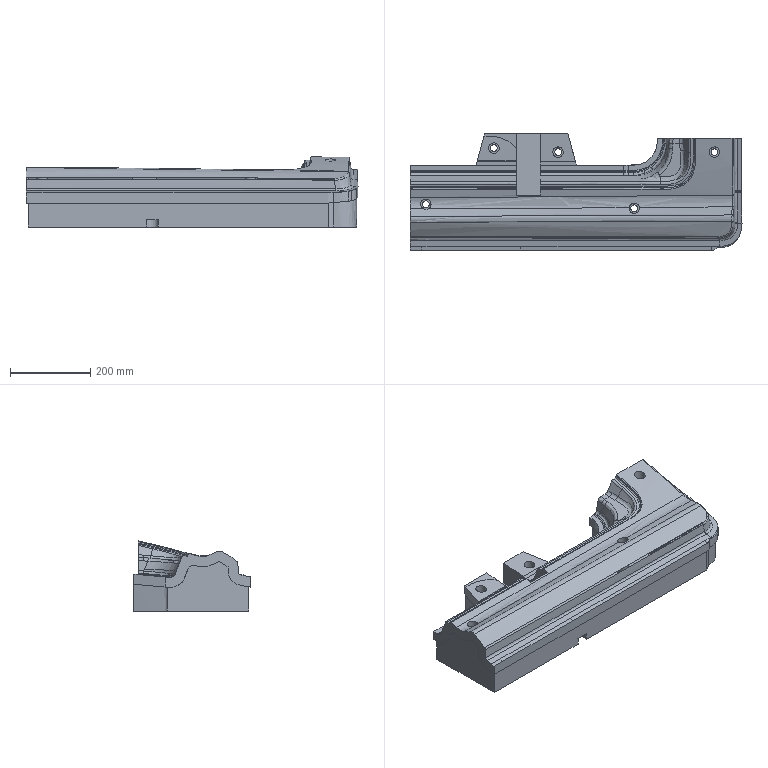Part | NX | features solid 2 | 1 solid | 194 faces | box 828.337 x 291.818 x 174.878 mm | volume 23738544 mm3 | spline 150 | plane 28 | cylinder 16 | commonest cylinder face diameters 32 x6 17 x5 26 x5